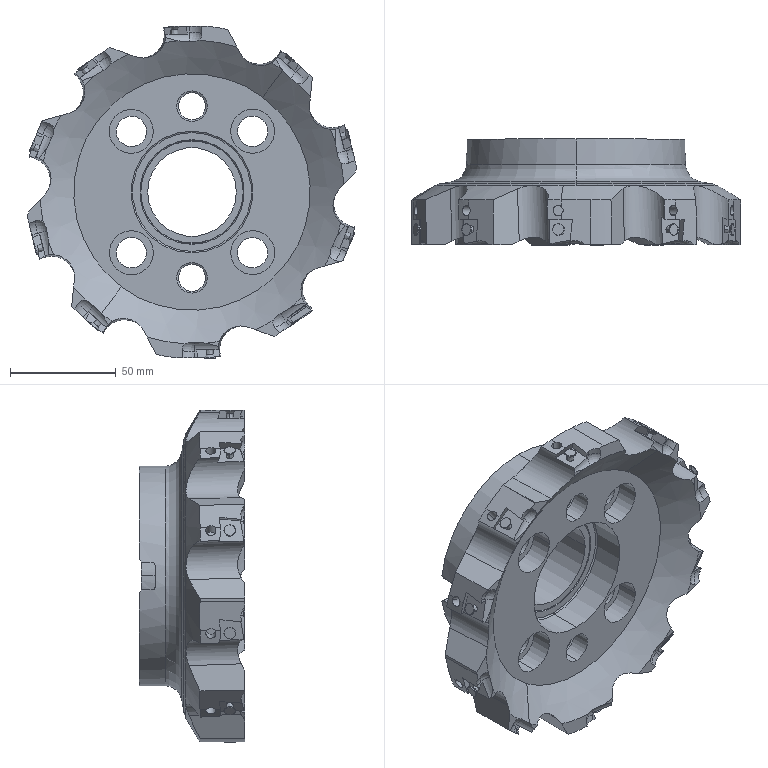Part | SolidWorks | features BaseBody 1 | 1 solid | 370 faces | box 156.206 x 50.016 x 157.229 mm | volume 398848 mm3 | plane 153 | cylinder 110 | cone 55 | torus 34 | spline 18 | commonest cylinder face diameters 4.8 x20 157.6 x16 12.8 x14 14.4 x12 9.6 x10 21.6 x10